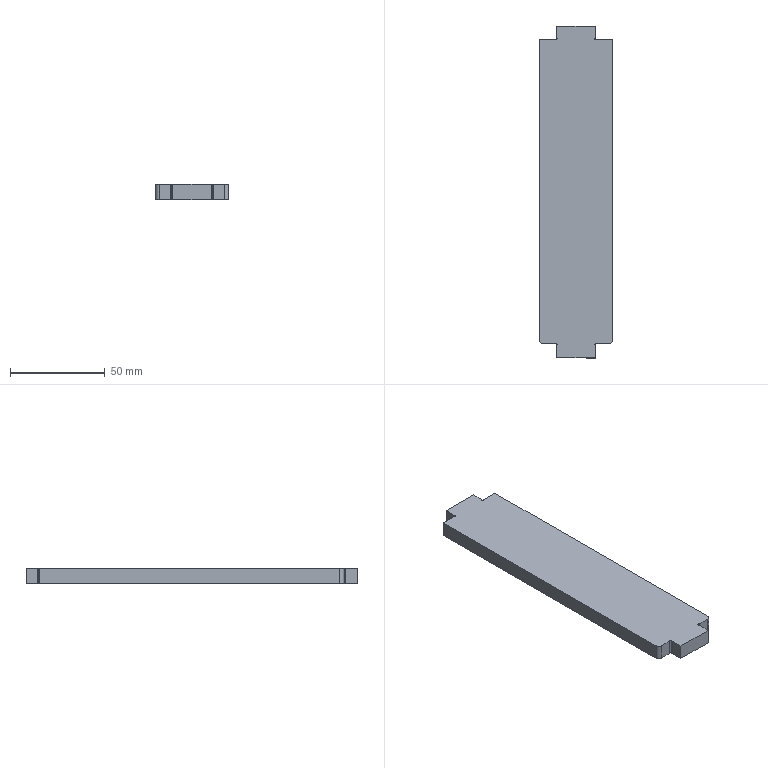Part | SolidWorks | features Fillet 2, FlatPattern 1, ICE 1, SMBaseFlange 1, SheetMetal 1 | 1 solid | 30 faces | box 38.5 x 175.3 x 8 mm | volume 51881 mm3 | cylinder 16 | plane 14 | commonest cylinder face diameters 2 x8 1 x6 4 x2
STEP:
#1=CARTESIAN_POINT('',(110.607,-414.685,0.));
#2=VERTEX_POINT('',#1);
#3=CARTESIAN_POINT('',(109.831,-415.102,0.));
#4=VERTEX_POINT('',#3);
#5=CARTESIAN_POINT('',(110.331,-415.102,0.));
#6=DIRECTION('',(0.,0.,1.));
#7=DIRECTION('',(1.,0.,0.));
#8=AXIS2_PLACEMENT_3D('',#5,#6,#7);
#9=CIRCLE('',#8,0.5);
#10=EDGE_CURVE('',#2,#4,#9,.T.);
#11=ORIENTED_EDGE('',*,*,#10,.T.);
#12=CARTESIAN_POINT('',(109.831,-415.102,-8.));
#13=VERTEX_POINT('',#12);
#14=CARTESIAN_POINT('',(109.831,-415.102,-8.));
#15=DIRECTION('',(0.,0.,-1.));
#16=VECTOR('',#15,1000.);
#17=LINE('',#14,#16);
#18=EDGE_CURVE('',#4,#13,#17,.T.);
#19=ORIENTED_EDGE('',*,*,#18,.T.);
#20=CARTESIAN_POINT('',(110.607,-414.685,-8.));
#21=VERTEX_POINT('',#20);
#22=CARTESIAN_POINT('',(110.331,-415.102,-8.));
#23=DIRECTION('',(0.,0.,1.));
#24=DIRECTION('',(1.,0.,0.));
#25=AXIS2_PLACEMENT_3D('',#22,#23,#24);
#26=CIRCLE('',#25,0.5);
#27=EDGE_CURVE('',#21,#13,#26,.T.);
#28=ORIENTED_EDGE('',*,*,#27,.F.);
#29=CARTESIAN_POINT('',(110.607,-414.685,-8.));
#30=DIRECTION('',(0.,0.,1.));
#31=VECTOR('',#30,1000.);
#32=LINE('',#29,#31);
#33=EDGE_CURVE('',#21,#2,#32,.T.);
#34=ORIENTED_EDGE('',*,*,#33,.T.);
#35=EDGE_LOOP('',(#11,#19,#28,#34));
#36=FACE_OUTER_BOUND('',#35,.T.);
#37=CARTESIAN_POINT('',(110.331,-415.102,-8.));
#38=DIRECTION('',(0.,0.,-1.));
#39=DIRECTION('',(-1.,0.,0.));
#40=AXIS2_PLACEMENT_3D('',#37,#38,#39);
#41=CYLINDRICAL_SURFACE('',#40,0.5);
#42=ADVANCED_FACE('',(#36),#41,.F.);
#43=CARTESIAN_POINT('',(109.914,-253.526,0.));
#44=VERTEX_POINT('',#43);
#45=CARTESIAN_POINT('',(109.831,-253.802,0.));
#46=VERTEX_POINT('',#45);
#47=CARTESIAN_POINT('',(110.331,-253.802,0.));
#48=DIRECTION('',(0.,0.,1.));
#49=DIRECTION('',(1.,0.,0.));
#50=AXIS2_PLACEMENT_3D('',#47,#48,#49);
#51=CIRCLE('',#50,0.5);
#52=EDGE_CURVE('',#44,#46,#51,.T.);
#53=ORIENTED_EDGE('',*,*,#52,.T.);
#54=CARTESIAN_POINT('',(109.831,-253.802,-8.));
#55=VERTEX_POINT('',#54);
#56=CARTESIAN_POINT('',(109.831,-253.802,-8.));
#57=DIRECTION('',(0.,0.,-1.));
#58=VECTOR('',#57,1000.);
#59=LINE('',#56,#58);
#60=EDGE_CURVE('',#46,#55,#59,.T.);
#61=ORIENTED_EDGE('',*,*,#60,.T.);
#62=CARTESIAN_POINT('',(109.914,-253.526,-8.));
#63=VERTEX_POINT('',#62);
#64=CARTESIAN_POINT('',(110.331,-253.802,-8.));
#65=DIRECTION('',(0.,0.,1.));
#66=DIRECTION('',(1.,0.,0.));
#67=AXIS2_PLACEMENT_3D('',#64,#65,#66);
#68=CIRCLE('',#67,0.5);
#69=EDGE_CURVE('',#63,#55,#68,.T.);
#70=ORIENTED_EDGE('',*,*,#69,.F.);
#71=CARTESIAN_POINT('',(109.914,-253.526,-8.));
#72=DIRECTION('',(0.,0.,1.));
#73=VECTOR('',#72,1000.);
#74=LINE('',#71,#73);
#75=EDGE_CURVE('',#63,#44,#74,.T.);
#76=ORIENTED_EDGE('',*,*,#75,.T.);
#77=EDGE_LOOP('',(#53,#61,#70,#76));
#78=FACE_OUTER_BOUND('',#77,.T.);
#79=CARTESIAN_POINT('',(110.331,-253.802,-8.));
#80=DIRECTION('',(0.,0.,-1.));
#81=DIRECTION('',(-1.,0.,0.));
#82=AXIS2_PLACEMENT_3D('',#79,#80,#81);
#83=CYLINDRICAL_SURFACE('',#82,0.5);
#84=ADVANCED_FACE('',(#78),#83,.F.);
#85=CARTESIAN_POINT('',(82.581,-414.852,0.));
#86=VERTEX_POINT('',#85);
#87=CARTESIAN_POINT('',(88.502,-414.852,0.));
#88=VERTEX_POINT('',#87);
#89=CARTESIAN_POINT('',(80.581,-414.852,0.));
#90=DIRECTION('',(1.,0.,0.));
#91=VECTOR('',#90,1000.);
#92=LINE('',#89,#91);
#93=EDGE_CURVE('',#86,#88,#92,.T.);
#94=ORIENTED_EDGE('',*,*,#93,.F.);
#95=CARTESIAN_POINT('',(82.581,-414.852,-8.));
#96=VERTEX_POINT('',#95);
#97=CARTESIAN_POINT('',(82.581,-414.852,-8.));
#98=DIRECTION('',(0.,0.,-1.));
#99=VECTOR('',#98,1000.);
#100=LINE('',#97,#99);
#101=EDGE_CURVE('',#86,#96,#100,.T.);
#102=ORIENTED_EDGE('',*,*,#101,.T.);
#103=CARTESIAN_POINT('',(88.502,-414.852,-8.));
#104=VERTEX_POINT('',#103);
#105=CARTESIAN_POINT('',(80.581,-414.852,-8.));
#106=DIRECTION('',(1.,0.,0.));
#107=VECTOR('',#106,1000.);
#108=LINE('',#105,#107);
#109=EDGE_CURVE('',#96,#104,#108,.T.);
#110=ORIENTED_EDGE('',*,*,#109,.T.);
#111=CARTESIAN_POINT('',(88.502,-414.852,-8.));
#112=DIRECTION('',(0.,0.,1.));
#113=VECTOR('',#112,1000.);
#114=LINE('',#111,#113);
#115=EDGE_CURVE('',#104,#88,#114,.T.);
#116=ORIENTED_EDGE('',*,*,#115,.T.);
#117=EDGE_LOOP('',(#94,#102,#110,#116));
#118=FACE_OUTER_BOUND('',#117,.T.);
#119=CARTESIAN_POINT('',(80.581,-414.852,-8.));
#120=DIRECTION('',(0.,-1.,0.));
#121=DIRECTION('',(1.,0.,0.));
#122=AXIS2_PLACEMENT_3D('',#119,#120,#121);
#123=PLANE('',#122);
#124=ADVANCED_FACE('',(#118),#123,.T.);
#125=CARTESIAN_POINT('',(88.502,-254.052,0.));
#126=VERTEX_POINT('',#125);
#127=CARTESIAN_POINT('',(80.581,-254.052,0.));
#128=VERTEX_POINT('',#127);
#129=CARTESIAN_POINT('',(80.581,-254.052,0.));
#130=DIRECTION('',(-1.,0.,0.));
#131=VECTOR('',#130,1000.);
#132=LINE('',#129,#131);
#133=EDGE_CURVE('',#126,#128,#132,.T.);
#134=ORIENTED_EDGE('',*,*,#133,.F.);
#135=CARTESIAN_POINT('',(88.502,-254.052,-8.));
#136=VERTEX_POINT('',#135);
#137=CARTESIAN_POINT('',(88.502,-254.052,-8.));
#138=DIRECTION('',(0.,0.,-1.));
#139=VECTOR('',#138,1000.);
#140=LINE('',#137,#139);
#141=EDGE_CURVE('',#126,#136,#140,.T.);
#142=ORIENTED_EDGE('',*,*,#141,.T.);
#143=CARTESIAN_POINT('',(80.581,-254.052,-8.));
#144=VERTEX_POINT('',#143);
#145=CARTESIAN_POINT('',(80.581,-254.052,-8.));
#146=DIRECTION('',(-1.,0.,0.));
#147=VECTOR('',#146,1000.);
#148=LINE('',#145,#147);
#149=EDGE_CURVE('',#136,#144,#148,.T.);
#150=ORIENTED_EDGE('',*,*,#149,.T.);
#151=CARTESIAN_POINT('',(80.581,-254.052,-8.));
#152=DIRECTION('',(0.,0.,1.));
#153=VECTOR('',#152,1000.);
#154=LINE('',#151,#153);
#155=EDGE_CURVE('',#144,#128,#154,.T.);
#156=ORIENTED_EDGE('',*,*,#155,.T.);
#157=EDGE_LOOP('',(#134,#142,#150,#156));
#158=FACE_OUTER_BOUND('',#157,.T.);
#159=CARTESIAN_POINT('',(80.581,-254.052,-8.));
#160=DIRECTION('',(0.,1.,0.));
#161=DIRECTION('',(0.,0.,1.));
#162=AXIS2_PLACEMENT_3D('',#159,#160,#161);
#163=PLANE('',#162);
#164=ADVANCED_FACE('',(#158),#163,.T.);
#165=CARTESIAN_POINT('',(89.581,-247.052,-8.));
#166=VERTEX_POINT('',#165);
#167=CARTESIAN_POINT('',(89.581,-252.973,-8.));
#168=VERTEX_POINT('',#167);
#169=CARTESIAN_POINT('',(89.581,-254.052,-8.));
#170=DIRECTION('',(0.,-1.,0.));
#171=VECTOR('',#170,1000.);
#172=LINE('',#169,#171);
#173=EDGE_CURVE('',#166,#168,#172,.T.);
#174=ORIENTED_EDGE('',*,*,#173,.T.);
#175=CARTESIAN_POINT('',(89.581,-252.973,0.));
#176=VERTEX_POINT('',#175);
#177=CARTESIAN_POINT('',(89.581,-252.973,-8.));
#178=DIRECTION('',(0.,0.,1.));
#179=VECTOR('',#178,1000.);
#180=LINE('',#177,#179);
#181=EDGE_CURVE('',#168,#176,#180,.T.);
#182=ORIENTED_EDGE('',*,*,#181,.T.);
#183=CARTESIAN_POINT('',(89.581,-247.052,0.));
#184=VERTEX_POINT('',#183);
#185=CARTESIAN_POINT('',(89.581,-254.052,0.));
#186=DIRECTION('',(0.,-1.,0.));
#187=VECTOR('',#186,1000.);
#188=LINE('',#185,#187);
#189=EDGE_CURVE('',#184,#176,#188,.T.);
#190=ORIENTED_EDGE('',*,*,#189,.F.);
#191=CARTESIAN_POINT('',(89.581,-247.052,-8.));
#192=DIRECTION('',(0.,0.,1.));
#193=VECTOR('',#192,1000.);
#194=LINE('',#191,#193);
#195=EDGE_CURVE('',#166,#184,#194,.T.);
#196=ORIENTED_EDGE('',*,*,#195,.F.);
#197=EDGE_LOOP('',(#174,#182,#190,#196));
#198=FACE_OUTER_BOUND('',#197,.T.);
#199=CARTESIAN_POINT('',(89.581,-254.052,-8.));
#200=DIRECTION('',(-1.,0.,0.));
#201=DIRECTION('',(0.,0.,1.));
#202=AXIS2_PLACEMENT_3D('',#199,#200,#201);
#203=PLANE('',#202);
#204=ADVANCED_FACE('',(#198),#203,.T.);
#205=CARTESIAN_POINT('',(110.081,-252.973,0.));
#206=VERTEX_POINT('',#205);
#207=CARTESIAN_POINT('',(110.081,-247.052,0.));
#208=VERTEX_POINT('',#207);
#209=CARTESIAN_POINT('',(110.081,-247.052,0.));
#210=DIRECTION('',(0.,1.,0.));
#211=VECTOR('',#210,1000.);
#212=LINE('',#209,#211);
#213=EDGE_CURVE('',#206,#208,#212,.T.);
#214=ORIENTED_EDGE('',*,*,#213,.F.);
#215=CARTESIAN_POINT('',(110.081,-252.973,-8.));
#216=VERTEX_POINT('',#215);
#217=CARTESIAN_POINT('',(110.081,-252.973,-8.));
#218=DIRECTION('',(0.,0.,-1.));
#219=VECTOR('',#218,1000.);
#220=LINE('',#217,#219);
#221=EDGE_CURVE('',#206,#216,#220,.T.);
#222=ORIENTED_EDGE('',*,*,#221,.T.);
#223=CARTESIAN_POINT('',(110.081,-247.052,-8.));
#224=VERTEX_POINT('',#223);
#225=CARTESIAN_POINT('',(110.081,-247.052,-8.));
#226=DIRECTION('',(0.,1.,0.));
#227=VECTOR('',#226,1000.);
#228=LINE('',#225,#227);
#229=EDGE_CURVE('',#216,#224,#228,.T.);
#230=ORIENTED_EDGE('',*,*,#229,.T.);
#231=CARTESIAN_POINT('',(110.081,-247.052,-8.));
#232=DIRECTION('',(0.,0.,1.));
#233=VECTOR('',#232,1000.);
#234=LINE('',#231,#233);
#235=EDGE_CURVE('',#224,#208,#234,.T.);
#236=ORIENTED_EDGE('',*,*,#235,.T.);
#237=EDGE_LOOP('',(#214,#222,#230,#236));
#238=FACE_OUTER_BOUND('',#237,.T.);
#239=CARTESIAN_POINT('',(110.081,-247.052,-8.));
#240=DIRECTION('',(1.,0.,0.));
#241=DIRECTION('',(0.,0.,-1.));
#242=AXIS2_PLACEMENT_3D('',#239,#240,#241);
#243=PLANE('',#242);
#244=ADVANCED_FACE('',(#238),#243,.T.);
#245=CARTESIAN_POINT('',(119.081,-254.052,-8.));
#246=VERTEX_POINT('',#245);
#247=CARTESIAN_POINT('',(111.16,-254.052,-8.));
#248=VERTEX_POINT('',#247);
#249=CARTESIAN_POINT('',(110.081,-254.052,-8.));
#250=DIRECTION('',(-1.,0.,0.));
#251=VECTOR('',#250,1000.);
#252=LINE('',#249,#251);
#253=EDGE_CURVE('',#246,#248,#252,.T.);
#254=ORIENTED_EDGE('',*,*,#253,.T.);
#255=CARTESIAN_POINT('',(111.16,-254.052,0.));
#256=VERTEX_POINT('',#255);
#257=CARTESIAN_POINT('',(111.16,-254.052,-8.));
#258=DIRECTION('',(0.,0.,1.));
#259=VECTOR('',#258,1000.);
#260=LINE('',#257,#259);
#261=EDGE_CURVE('',#248,#256,#260,.T.);
#262=ORIENTED_EDGE('',*,*,#261,.T.);
#263=CARTESIAN_POINT('',(119.081,-254.052,0.));
#264=VERTEX_POINT('',#263);
#265=CARTESIAN_POINT('',(110.081,-254.052,0.));
#266=DIRECTION('',(-1.,0.,0.));
#267=VECTOR('',#266,1000.);
#268=LINE('',#265,#267);
#269=EDGE_CURVE('',#264,#256,#268,.T.);
#270=ORIENTED_EDGE('',*,*,#269,.F.);
#271=CARTESIAN_POINT('',(119.081,-254.052,-8.));
#272=DIRECTION('',(0.,0.,1.));
#273=VECTOR('',#272,1000.);
#274=LINE('',#271,#273);
#275=EDGE_CURVE('',#246,#264,#274,.T.);
#276=ORIENTED_EDGE('',*,*,#275,.F.);
#277=EDGE_LOOP('',(#254,#262,#270,#276));
#278=FACE_OUTER_BOUND('',#277,.T.);
#279=CARTESIAN_POINT('',(110.081,-254.052,-8.));
#280=DIRECTION('',(0.,1.,0.));
#281=DIRECTION('',(0.,0.,1.));
#282=AXIS2_PLACEMENT_3D('',#279,#280,#281);
#283=PLANE('',#282);
#284=ADVANCED_FACE('',(#278),#283,.T.);
#285=CARTESIAN_POINT('',(111.16,-414.852,-8.));
#286=VERTEX_POINT('',#285);
#287=CARTESIAN_POINT('',(117.081,-414.852,-8.));
#288=VERTEX_POINT('',#287);
#289=CARTESIAN_POINT('',(110.081,-414.852,-8.));
#290=DIRECTION('',(1.,0.,0.));
#291=VECTOR('',#290,1000.);
#292=LINE('',#289,#291);
#293=EDGE_CURVE('',#286,#288,#292,.T.);
#294=ORIENTED_EDGE('',*,*,#293,.T.);
#295=CARTESIAN_POINT('',(117.081,-414.852,0.));
#296=VERTEX_POINT('',#295);
#297=CARTESIAN_POINT('',(117.081,-414.852,-8.));
#298=DIRECTION('',(0.,0.,1.));
#299=VECTOR('',#298,1000.);
#300=LINE('',#297,#299);
#301=EDGE_CURVE('',#288,#296,#300,.T.);
#302=ORIENTED_EDGE('',*,*,#301,.T.);
#303=CARTESIAN_POINT('',(111.16,-414.852,0.));
#304=VERTEX_POINT('',#303);
#305=CARTESIAN_POINT('',(110.081,-414.852,0.));
#306=DIRECTION('',(1.,0.,0.));
#307=VECTOR('',#306,1000.);
#308=LINE('',#305,#307);
#309=EDGE_CURVE('',#304,#296,#308,.T.);
#310=ORIENTED_EDGE('',*,*,#309,.F.);
#311=CARTESIAN_POINT('',(111.16,-414.852,-8.));
#312=DIRECTION('',(0.,0.,-1.));
#313=VECTOR('',#312,1000.);
#314=LINE('',#311,#313);
#315=EDGE_CURVE('',#304,#286,#314,.T.);
#316=ORIENTED_EDGE('',*,*,#315,.T.);
#317=EDGE_LOOP('',(#294,#302,#310,#316));
#318=FACE_OUTER_BOUND('',#317,.T.);
#319=CARTESIAN_POINT('',(110.081,-414.852,-8.));
#320=DIRECTION('',(0.,-1.,0.));
#321=DIRECTION('',(1.,0.,0.));
#322=AXIS2_PLACEMENT_3D('',#319,#320,#321);
#323=PLANE('',#322);
#324=ADVANCED_FACE('',(#318),#323,.T.);
#325=CARTESIAN_POINT('',(110.081,-422.352,-8.));
#326=VERTEX_POINT('',#325);
#327=CARTESIAN_POINT('',(110.081,-415.931,-8.));
#328=VERTEX_POINT('',#327);
#329=CARTESIAN_POINT('',(110.081,-422.352,-8.));
#330=DIRECTION('',(0.,1.,0.));
#331=VECTOR('',#330,1000.);
#332=LINE('',#329,#331);
#333=EDGE_CURVE('',#326,#328,#332,.T.);
#334=ORIENTED_EDGE('',*,*,#333,.T.);
#335=CARTESIAN_POINT('',(110.081,-415.931,0.));
#336=VERTEX_POINT('',#335);
#337=CARTESIAN_POINT('',(110.081,-415.931,-8.));
#338=DIRECTION('',(0.,0.,1.));
#339=VECTOR('',#338,1000.);
#340=LINE('',#337,#339);
#341=EDGE_CURVE('',#328,#336,#340,.T.);
#342=ORIENTED_EDGE('',*,*,#341,.T.);
#343=CARTESIAN_POINT('',(110.081,-422.352,0.));
#344=VERTEX_POINT('',#343);
#345=CARTESIAN_POINT('',(110.081,-422.352,0.));
#346=DIRECTION('',(0.,1.,0.));
#347=VECTOR('',#346,1000.);
#348=LINE('',#345,#347);
#349=EDGE_CURVE('',#344,#336,#348,.T.);
#350=ORIENTED_EDGE('',*,*,#349,.F.);
#351=CARTESIAN_POINT('',(110.081,-422.352,-8.));
#352=DIRECTION('',(0.,0.,1.));
#353=VECTOR('',#352,1000.);
#354=LINE('',#351,#353);
#355=EDGE_CURVE('',#326,#344,#354,.T.);
#356=ORIENTED_EDGE('',*,*,#355,.F.);
#357=EDGE_LOOP('',(#334,#342,#350,#356));
#358=FACE_OUTER_BOUND('',#357,.T.);
#359=CARTESIAN_POINT('',(110.081,-422.352,-8.));
#360=DIRECTION('',(1.,0.,0.));
#361=DIRECTION('',(0.,0.,-1.));
#362=AXIS2_PLACEMENT_3D('',#359,#360,#361);
#363=PLANE('',#362);
#364=ADVANCED_FACE('',(#358),#363,.T.);
#365=CARTESIAN_POINT('',(89.581,-415.931,0.));
#366=VERTEX_POINT('',#365);
#367=CARTESIAN_POINT('',(89.581,-422.352,0.));
#368=VERTEX_POINT('',#367);
#369=CARTESIAN_POINT('',(89.581,-414.852,0.));
#370=DIRECTION('',(0.,-1.,0.));
#371=VECTOR('',#370,1000.);
#372=LINE('',#369,#371);
#373=EDGE_CURVE('',#366,#368,#372,.T.);
#374=ORIENTED_EDGE('',*,*,#373,.F.);
#375=CARTESIAN_POINT('',(89.581,-415.931,-8.));
#376=VERTEX_POINT('',#375);
#377=CARTESIAN_POINT('',(89.581,-415.931,-8.));
#378=DIRECTION('',(0.,0.,-1.));
#379=VECTOR('',#378,1000.);
#380=LINE('',#377,#379);
#381=EDGE_CURVE('',#366,#376,#380,.T.);
#382=ORIENTED_EDGE('',*,*,#381,.T.);
#383=CARTESIAN_POINT('',(89.581,-422.352,-8.));
#384=VERTEX_POINT('',#383);
#385=CARTESIAN_POINT('',(89.581,-414.852,-8.));
#386=DIRECTION('',(0.,-1.,0.));
#387=VECTOR('',#386,1000.);
#388=LINE('',#385,#387);
#389=EDGE_CURVE('',#376,#384,#388,.T.);
#390=ORIENTED_EDGE('',*,*,#389,.T.);
#391=CARTESIAN_POINT('',(89.581,-422.352,-8.));
#392=DIRECTION('',(0.,0.,1.));
#393=VECTOR('',#392,1000.);
#394=LINE('',#391,#393);
#395=EDGE_CURVE('',#384,#368,#394,.T.);
#396=ORIENTED_EDGE('',*,*,#395,.T.);
#397=EDGE_LOOP('',(#374,#382,#390,#396));
#398=FACE_OUTER_BOUND('',#397,.T.);
#399=CARTESIAN_POINT('',(89.581,-414.852,-8.));
#400=DIRECTION('',(-1.,0.,0.));
#401=DIRECTION('',(0.,-1.,0.));
#402=AXIS2_PLACEMENT_3D('',#399,#400,#401);
#403=PLANE('',#402);
#404=ADVANCED_FACE('',(#398),#403,.T.);
#405=CARTESIAN_POINT('',(119.081,-412.852,-8.));
#406=VERTEX_POINT('',#405);
#407=CARTESIAN_POINT('',(119.081,-254.052,-8.));
#408=DIRECTION('',(0.,1.,0.));
#409=VECTOR('',#408,1000.);
#410=LINE('',#407,#409);
#411=EDGE_CURVE('',#406,#246,#410,.T.);
#412=ORIENTED_EDGE('',*,*,#411,.F.);
#413=CARTESIAN_POINT('',(117.081,-412.852,-8.));
#414=DIRECTION('',(0.,0.,-1.));
#415=DIRECTION('',(-1.,0.,0.));
#416=AXIS2_PLACEMENT_3D('',#413,#414,#415);
#417=CIRCLE('',#416,2.);
#418=EDGE_CURVE('',#406,#288,#417,.T.);
#419=ORIENTED_EDGE('',*,*,#418,.T.);
#420=ORIENTED_EDGE('',*,*,#293,.F.);
#421=CARTESIAN_POINT('',(111.16,-413.852,-8.));
#422=DIRECTION('',(0.,0.,-1.));
#423=DIRECTION('',(-1.,0.,0.));
#424=AXIS2_PLACEMENT_3D('',#421,#422,#423);
#425=CIRCLE('',#424,1.);
#426=EDGE_CURVE('',#286,#21,#425,.T.);
#427=ORIENTED_EDGE('',*,*,#426,.T.);
#428=ORIENTED_EDGE('',*,*,#27,.T.);
#429=CARTESIAN_POINT('',(109.914,-415.378,-8.));
#430=VERTEX_POINT('',#429);
#431=CARTESIAN_POINT('',(110.331,-415.102,-8.));
#432=DIRECTION('',(0.,0.,1.));
#433=DIRECTION('',(1.,0.,0.));
#434=AXIS2_PLACEMENT_3D('',#431,#432,#433);
#435=CIRCLE('',#434,0.5);
#436=EDGE_CURVE('',#13,#430,#435,.T.);
#437=ORIENTED_EDGE('',*,*,#436,.T.);
#438=CARTESIAN_POINT('',(109.081,-415.931,-8.));
#439=DIRECTION('',(0.,0.,-1.));
#440=DIRECTION('',(-1.,0.,0.));
#441=AXIS2_PLACEMENT_3D('',#438,#439,#440);
#442=CIRCLE('',#441,1.);
#443=EDGE_CURVE('',#430,#328,#442,.T.);
#444=ORIENTED_EDGE('',*,*,#443,.T.);
#445=ORIENTED_EDGE('',*,*,#333,.F.);
#446=CARTESIAN_POINT('',(89.581,-422.352,-8.));
#447=DIRECTION('',(1.,0.,0.));
#448=VECTOR('',#447,1000.);
#449=LINE('',#446,#448);
#450=EDGE_CURVE('',#384,#326,#449,.T.);
#451=ORIENTED_EDGE('',*,*,#450,.F.);
#452=ORIENTED_EDGE('',*,*,#389,.F.);
#453=CARTESIAN_POINT('',(89.747,-415.378,-8.));
#454=VERTEX_POINT('',#453);
#455=CARTESIAN_POINT('',(90.581,-415.931,-8.));
#456=DIRECTION('',(0.,0.,-1.));
#457=DIRECTION('',(-1.,0.,0.));
#458=AXIS2_PLACEMENT_3D('',#455,#456,#457);
#459=CIRCLE('',#458,1.);
#460=EDGE_CURVE('',#376,#454,#459,.T.);
#461=ORIENTED_EDGE('',*,*,#460,.T.);
#462=CARTESIAN_POINT('',(89.054,-414.685,-8.));
#463=VERTEX_POINT('',#462);
#464=CARTESIAN_POINT('',(89.331,-415.102,-8.));
#465=DIRECTION('',(0.,0.,-1.));
#466=DIRECTION('',(-1.,0.,0.));
#467=AXIS2_PLACEMENT_3D('',#464,#465,#466);
#468=CIRCLE('',#467,0.5);
#469=EDGE_CURVE('',#463,#454,#468,.T.);
#470=ORIENTED_EDGE('',*,*,#469,.F.);
#471=CARTESIAN_POINT('',(88.502,-413.852,-8.));
#472=DIRECTION('',(0.,0.,-1.));
#473=DIRECTION('',(-1.,0.,0.));
#474=AXIS2_PLACEMENT_3D('',#471,#472,#473);
#475=CIRCLE('',#474,1.);
#476=EDGE_CURVE('',#463,#104,#475,.T.);
#477=ORIENTED_EDGE('',*,*,#476,.T.);
#478=ORIENTED_EDGE('',*,*,#109,.F.);
#479=CARTESIAN_POINT('',(80.581,-412.852,-8.));
#480=VERTEX_POINT('',#479);
#481=CARTESIAN_POINT('',(82.581,-412.852,-8.));
#482=DIRECTION('',(0.,0.,-1.));
#483=DIRECTION('',(-1.,0.,0.));
#484=AXIS2_PLACEMENT_3D('',#481,#482,#483);
#485=CIRCLE('',#484,2.);
#486=EDGE_CURVE('',#96,#480,#485,.T.);
#487=ORIENTED_EDGE('',*,*,#486,.T.);
#488=CARTESIAN_POINT('',(80.581,-414.852,-8.));
#489=DIRECTION('',(0.,-1.,0.));
#490=VECTOR('',#489,1000.);
#491=LINE('',#488,#490);
#492=EDGE_CURVE('',#144,#480,#491,.T.);
#493=ORIENTED_EDGE('',*,*,#492,.F.);
#494=ORIENTED_EDGE('',*,*,#149,.F.);
#495=CARTESIAN_POINT('',(89.054,-254.219,-8.));
#496=VERTEX_POINT('',#495);
#497=CARTESIAN_POINT('',(88.502,-255.052,-8.));
#498=DIRECTION('',(0.,0.,-1.));
#499=DIRECTION('',(-1.,0.,0.));
#500=AXIS2_PLACEMENT_3D('',#497,#498,#499);
#501=CIRCLE('',#500,1.);
#502=EDGE_CURVE('',#136,#496,#501,.T.);
#503=ORIENTED_EDGE('',*,*,#502,.T.);
#504=CARTESIAN_POINT('',(89.747,-253.526,-8.));
#505=VERTEX_POINT('',#504);
#506=CARTESIAN_POINT('',(89.331,-253.802,-8.));
#507=DIRECTION('',(0.,0.,1.));
#508=DIRECTION('',(1.,0.,0.));
#509=AXIS2_PLACEMENT_3D('',#506,#507,#508);
#510=CIRCLE('',#509,0.5);
#511=EDGE_CURVE('',#496,#505,#510,.T.);
#512=ORIENTED_EDGE('',*,*,#511,.T.);
#513=CARTESIAN_POINT('',(90.581,-252.973,-8.));
#514=DIRECTION('',(0.,0.,-1.));
#515=DIRECTION('',(-1.,0.,0.));
#516=AXIS2_PLACEMENT_3D('',#513,#514,#515);
#517=CIRCLE('',#516,1.);
#518=EDGE_CURVE('',#505,#168,#517,.T.);
#519=ORIENTED_EDGE('',*,*,#518,.T.);
#520=ORIENTED_EDGE('',*,*,#173,.F.);
#521=CARTESIAN_POINT('',(89.581,-247.052,-8.));
#522=DIRECTION('',(-1.,0.,0.));
#523=VECTOR('',#522,1000.);
#524=LINE('',#521,#523);
#525=EDGE_CURVE('',#224,#166,#524,.T.);
#526=ORIENTED_EDGE('',*,*,#525,.F.);
#527=ORIENTED_EDGE('',*,*,#229,.F.);
#528=CARTESIAN_POINT('',(109.081,-252.973,-8.));
#529=DIRECTION('',(0.,0.,-1.));
#530=DIRECTION('',(-1.,0.,0.));
#531=AXIS2_PLACEMENT_3D('',#528,#529,#530);
#532=CIRCLE('',#531,1.);
#533=EDGE_CURVE('',#216,#63,#532,.T.);
#534=ORIENTED_EDGE('',*,*,#533,.T.);
#535=ORIENTED_EDGE('',*,*,#69,.T.);
#536=CARTESIAN_POINT('',(110.607,-254.219,-8.));
#537=VERTEX_POINT('',#536);
#538=CARTESIAN_POINT('',(110.331,-253.802,-8.));
#539=DIRECTION('',(0.,0.,1.));
#540=DIRECTION('',(1.,0.,0.));
#541=AXIS2_PLACEMENT_3D('',#538,#539,#540);
#542=CIRCLE('',#541,0.5);
#543=EDGE_CURVE('',#55,#537,#542,.T.);
#544=ORIENTED_EDGE('',*,*,#543,.T.);
#545=CARTESIAN_POINT('',(111.16,-255.052,-8.));
#546=DIRECTION('',(0.,0.,-1.));
#547=DIRECTION('',(-1.,0.,0.));
#548=AXIS2_PLACEMENT_3D('',#545,#546,#547);
#549=CIRCLE('',#548,1.);
#550=EDGE_CURVE('',#537,#248,#549,.T.);
#551=ORIENTED_EDGE('',*,*,#550,.T.);
#552=ORIENTED_EDGE('',*,*,#253,.F.);
#553=EDGE_LOOP('',(#412,#419,#420,#427,#428,#437,#444,#445,#451,#452,#461,#470,#477,#478,#487,#493,#494,#503,#512,#519,#520,#526,#527,#534,#535,#544,#551,#552));
#554=FACE_OUTER_BOUND('',#553,.T.);
#555=CARTESIAN_POINT('',(0.,0.,-8.));
#556=DIRECTION('',(0.,0.,-1.));
#557=DIRECTION('',(-1.,0.,0.));
#558=AXIS2_PLACEMENT_3D('',#555,#556,#557);
#559=PLANE('',#558);
#560=ADVANCED_FACE('',(#554),#559,.T.);
#561=ORIENTED_EDGE('',*,*,#309,.T.);
#562=CARTESIAN_POINT('',(119.081,-412.852,0.));
#563=VERTEX_POINT('',#562);
#564=CARTESIAN_POINT('',(117.081,-412.852,0.));
#565=DIRECTION('',(0.,0.,1.));
#566=DIRECTION('',(-1.,0.,0.));
#567=AXIS2_PLACEMENT_3D('',#564,#565,#566);
#568=CIRCLE('',#567,2.);
#569=EDGE_CURVE('',#296,#563,#568,.T.);
#570=ORIENTED_EDGE('',*,*,#569,.T.);
#571=CARTESIAN_POINT('',(119.081,-254.052,0.));
#572=DIRECTION('',(0.,1.,0.));
#573=VECTOR('',#572,1000.);
#574=LINE('',#571,#573);
#575=EDGE_CURVE('',#563,#264,#574,.T.);
#576=ORIENTED_EDGE('',*,*,#575,.T.);
#577=ORIENTED_EDGE('',*,*,#269,.T.);
#578=CARTESIAN_POINT('',(110.607,-254.219,0.));
#579=VERTEX_POINT('',#578);
#580=CARTESIAN_POINT('',(111.16,-255.052,0.));
#581=DIRECTION('',(0.,0.,1.));
#582=DIRECTION('',(-1.,0.,0.));
#583=AXIS2_PLACEMENT_3D('',#580,#581,#582);
#584=CIRCLE('',#583,1.);
#585=EDGE_CURVE('',#256,#579,#584,.T.);
#586=ORIENTED_EDGE('',*,*,#585,.T.);
#587=CARTESIAN_POINT('',(110.331,-253.802,0.));
#588=DIRECTION('',(0.,0.,1.));
#589=DIRECTION('',(1.,0.,0.));
#590=AXIS2_PLACEMENT_3D('',#587,#588,#589);
#591=CIRCLE('',#590,0.5);
#592=EDGE_CURVE('',#46,#579,#591,.T.);
#593=ORIENTED_EDGE('',*,*,#592,.F.);
#594=ORIENTED_EDGE('',*,*,#52,.F.);
#595=CARTESIAN_POINT('',(109.081,-252.973,0.));
#596=DIRECTION('',(0.,0.,1.));
#597=DIRECTION('',(-1.,0.,0.));
#598=AXIS2_PLACEMENT_3D('',#595,#596,#597);
#599=CIRCLE('',#598,1.);
#600=EDGE_CURVE('',#44,#206,#599,.T.);
#601=ORIENTED_EDGE('',*,*,#600,.T.);
#602=ORIENTED_EDGE('',*,*,#213,.T.);
#603=CARTESIAN_POINT('',(89.581,-247.052,0.));
#604=DIRECTION('',(-1.,0.,0.));
#605=VECTOR('',#604,1000.);
#606=LINE('',#603,#605);
#607=EDGE_CURVE('',#208,#184,#606,.T.);
#608=ORIENTED_EDGE('',*,*,#607,.T.);
#609=ORIENTED_EDGE('',*,*,#189,.T.);
#610=CARTESIAN_POINT('',(89.747,-253.526,0.));
#611=VERTEX_POINT('',#610);
#612=CARTESIAN_POINT('',(90.581,-252.973,0.));
#613=DIRECTION('',(0.,0.,1.));
#614=DIRECTION('',(-1.,0.,0.));
#615=AXIS2_PLACEMENT_3D('',#612,#613,#614);
#616=CIRCLE('',#615,1.);
#617=EDGE_CURVE('',#176,#611,#616,.T.);
#618=ORIENTED_EDGE('',*,*,#617,.T.);
#619=CARTESIAN_POINT('',(89.054,-254.219,0.));
#620=VERTEX_POINT('',#619);
#621=CARTESIAN_POINT('',(89.331,-253.802,0.));
#622=DIRECTION('',(0.,0.,1.));
#623=DIRECTION('',(1.,0.,0.));
#624=AXIS2_PLACEMENT_3D('',#621,#622,#623);
#625=CIRCLE('',#624,0.5);
#626=EDGE_CURVE('',#620,#611,#625,.T.);
#627=ORIENTED_EDGE('',*,*,#626,.F.);
#628=CARTESIAN_POINT('',(88.502,-255.052,0.));
#629=DIRECTION('',(0.,0.,1.));
#630=DIRECTION('',(-1.,0.,0.));
#631=AXIS2_PLACEMENT_3D('',#628,#629,#630);
#632=CIRCLE('',#631,1.);
#633=EDGE_CURVE('',#620,#126,#632,.T.);
#634=ORIENTED_EDGE('',*,*,#633,.T.);
#635=ORIENTED_EDGE('',*,*,#133,.T.);
#636=CARTESIAN_POINT('',(80.581,-412.852,0.));
#637=VERTEX_POINT('',#636);
#638=CARTESIAN_POINT('',(80.581,-414.852,0.));
#639=DIRECTION('',(0.,-1.,0.));
#640=VECTOR('',#639,1000.);
#641=LINE('',#638,#640);
#642=EDGE_CURVE('',#128,#637,#641,.T.);
#643=ORIENTED_EDGE('',*,*,#642,.T.);
#644=CARTESIAN_POINT('',(82.581,-412.852,0.));
#645=DIRECTION('',(0.,0.,1.));
#646=DIRECTION('',(-1.,0.,0.));
#647=AXIS2_PLACEMENT_3D('',#644,#645,#646);
#648=CIRCLE('',#647,2.);
#649=EDGE_CURVE('',#637,#86,#648,.T.);
#650=ORIENTED_EDGE('',*,*,#649,.T.);
#651=ORIENTED_EDGE('',*,*,#93,.T.);
#652=CARTESIAN_POINT('',(89.054,-414.685,0.));
#653=VERTEX_POINT('',#652);
#654=CARTESIAN_POINT('',(88.502,-413.852,0.));
#655=DIRECTION('',(0.,0.,1.));
#656=DIRECTION('',(-1.,0.,0.));
#657=AXIS2_PLACEMENT_3D('',#654,#655,#656);
#658=CIRCLE('',#657,1.);
#659=EDGE_CURVE('',#88,#653,#658,.T.);
#660=ORIENTED_EDGE('',*,*,#659,.T.);
#661=CARTESIAN_POINT('',(89.747,-415.378,0.));
#662=VERTEX_POINT('',#661);
#663=CARTESIAN_POINT('',(89.331,-415.102,0.));
#664=DIRECTION('',(0.,0.,-1.));
#665=DIRECTION('',(-1.,0.,0.));
#666=AXIS2_PLACEMENT_3D('',#663,#664,#665);
#667=CIRCLE('',#666,0.5);
#668=EDGE_CURVE('',#653,#662,#667,.T.);
#669=ORIENTED_EDGE('',*,*,#668,.T.);
#670=CARTESIAN_POINT('',(90.581,-415.931,0.));
#671=DIRECTION('',(0.,0.,1.));
#672=DIRECTION('',(-1.,0.,0.));
#673=AXIS2_PLACEMENT_3D('',#670,#671,#672);
#674=CIRCLE('',#673,1.);
#675=EDGE_CURVE('',#662,#366,#674,.T.);
#676=ORIENTED_EDGE('',*,*,#675,.T.);
#677=ORIENTED_EDGE('',*,*,#373,.T.);
#678=CARTESIAN_POINT('',(89.581,-422.352,0.));
#679=DIRECTION('',(1.,0.,0.));
#680=VECTOR('',#679,1000.);
#681=LINE('',#678,#680);
#682=EDGE_CURVE('',#368,#344,#681,.T.);
#683=ORIENTED_EDGE('',*,*,#682,.T.);
#684=ORIENTED_EDGE('',*,*,#349,.T.);
#685=CARTESIAN_POINT('',(109.914,-415.378,0.));
#686=VERTEX_POINT('',#685);
#687=CARTESIAN_POINT('',(109.081,-415.931,0.));
#688=DIRECTION('',(0.,0.,1.));
#689=DIRECTION('',(-1.,0.,0.));
#690=AXIS2_PLACEMENT_3D('',#687,#688,#689);
#691=CIRCLE('',#690,1.);
#692=EDGE_CURVE('',#336,#686,#691,.T.);
#693=ORIENTED_EDGE('',*,*,#692,.T.);
#694=CARTESIAN_POINT('',(110.331,-415.102,0.));
#695=DIRECTION('',(0.,0.,1.));
#696=DIRECTION('',(1.,0.,0.));
#697=AXIS2_PLACEMENT_3D('',#694,#695,#696);
#698=CIRCLE('',#697,0.5);
#699=EDGE_CURVE('',#4,#686,#698,.T.);
#700=ORIENTED_EDGE('',*,*,#699,.F.);
#701=ORIENTED_EDGE('',*,*,#10,.F.);
#702=CARTESIAN_POINT('',(111.16,-413.852,0.));
#703=DIRECTION('',(0.,0.,1.));
#704=DIRECTION('',(-1.,0.,0.));
#705=AXIS2_PLACEMENT_3D('',#702,#703,#704);
#706=CIRCLE('',#705,1.);
#707=EDGE_CURVE('',#2,#304,#706,.T.);
#708=ORIENTED_EDGE('',*,*,#707,.T.);
#709=EDGE_LOOP('',(#561,#570,#576,#577,#586,#593,#594,#601,#602,#608,#609,#618,#627,#634,#635,#643,#650,#651,#660,#669,#676,#677,#683,#684,#693,#700,#701,#708));
#710=FACE_OUTER_BOUND('',#709,.T.);
#711=CARTESIAN_POINT('',(0.,0.,0.));
#712=DIRECTION('',(0.,0.,-1.));
#713=DIRECTION('',(-1.,0.,0.));
#714=AXIS2_PLACEMENT_3D('',#711,#712,#713);
#715=PLANE('',#714);
#716=ADVANCED_FACE('',(#710),#715,.F.);
#717=ORIENTED_EDGE('',*,*,#492,.T.);
#718=CARTESIAN_POINT('',(80.581,-412.852,-8.));
#719=DIRECTION('',(0.,0.,1.));
#720=VECTOR('',#719,1000.);
#721=LINE('',#718,#720);
#722=EDGE_CURVE('',#480,#637,#721,.T.);
#723=ORIENTED_EDGE('',*,*,#722,.T.);
#724=ORIENTED_EDGE('',*,*,#642,.F.);
#725=ORIENTED_EDGE('',*,*,#155,.F.);
#726=EDGE_LOOP('',(#717,#723,#724,#725));
#727=FACE_OUTER_BOUND('',#726,.T.);
#728=CARTESIAN_POINT('',(80.581,-414.852,-8.));
#729=DIRECTION('',(-1.,0.,0.));
#730=DIRECTION('',(0.,-1.,0.));
#731=AXIS2_PLACEMENT_3D('',#728,#729,#730);
#732=PLANE('',#731);
#733=ADVANCED_FACE('',(#727),#732,.T.);
#734=ORIENTED_EDGE('',*,*,#607,.F.);
#735=ORIENTED_EDGE('',*,*,#235,.F.);
#736=ORIENTED_EDGE('',*,*,#525,.T.);
#737=ORIENTED_EDGE('',*,*,#195,.T.);
#738=EDGE_LOOP('',(#734,#735,#736,#737));
#739=FACE_OUTER_BOUND('',#738,.T.);
#740=CARTESIAN_POINT('',(89.581,-247.052,-8.));
#741=DIRECTION('',(0.,1.,0.));
#742=DIRECTION('',(0.,0.,1.));
#743=AXIS2_PLACEMENT_3D('',#740,#741,#742);
#744=PLANE('',#743);
#745=ADVANCED_FACE('',(#739),#744,.T.);
#746=ORIENTED_EDGE('',*,*,#575,.F.);
#747=CARTESIAN_POINT('',(119.081,-412.852,-8.));
#748=DIRECTION('',(0.,0.,-1.));
#749=VECTOR('',#748,1000.);
#750=LINE('',#747,#749);
#751=EDGE_CURVE('',#563,#406,#750,.T.);
#752=ORIENTED_EDGE('',*,*,#751,.T.);
#753=ORIENTED_EDGE('',*,*,#411,.T.);
#754=ORIENTED_EDGE('',*,*,#275,.T.);
#755=EDGE_LOOP('',(#746,#752,#753,#754));
#756=FACE_OUTER_BOUND('',#755,.T.);
#757=CARTESIAN_POINT('',(119.081,-254.052,-8.));
#758=DIRECTION('',(1.,0.,0.));
#759=DIRECTION('',(0.,1.,0.));
#760=AXIS2_PLACEMENT_3D('',#757,#758,#759);
#761=PLANE('',#760);
#762=ADVANCED_FACE('',(#756),#761,.T.);
#763=ORIENTED_EDGE('',*,*,#682,.F.);
#764=ORIENTED_EDGE('',*,*,#395,.F.);
#765=ORIENTED_EDGE('',*,*,#450,.T.);
#766=ORIENTED_EDGE('',*,*,#355,.T.);
#767=EDGE_LOOP('',(#763,#764,#765,#766));
#768=FACE_OUTER_BOUND('',#767,.T.);
#769=CARTESIAN_POINT('',(89.581,-422.352,-8.));
#770=DIRECTION('',(0.,-1.,0.));
#771=DIRECTION('',(1.,0.,0.));
#772=AXIS2_PLACEMENT_3D('',#769,#770,#771);
#773=PLANE('',#772);
#774=ADVANCED_FACE('',(#768),#773,.T.);
#775=ORIENTED_EDGE('',*,*,#668,.F.);
#776=CARTESIAN_POINT('',(89.054,-414.685,0.));
#777=DIRECTION('',(0.,0.,-1.));
#778=VECTOR('',#777,1000.);
#779=LINE('',#776,#778);
#780=EDGE_CURVE('',#653,#463,#779,.T.);
#781=ORIENTED_EDGE('',*,*,#780,.T.);
#782=ORIENTED_EDGE('',*,*,#469,.T.);
#783=CARTESIAN_POINT('',(89.747,-415.378,0.));
#784=DIRECTION('',(0.,0.,1.));
#785=VECTOR('',#784,1000.);
#786=LINE('',#783,#785);
#787=EDGE_CURVE('',#454,#662,#786,.T.);
#788=ORIENTED_EDGE('',*,*,#787,.T.);
#789=EDGE_LOOP('',(#775,#781,#782,#788));
#790=FACE_OUTER_BOUND('',#789,.T.);
#791=CARTESIAN_POINT('',(89.331,-415.102,0.));
#792=DIRECTION('',(0.,0.,-1.));
#793=DIRECTION('',(-1.,0.,0.));
#794=AXIS2_PLACEMENT_3D('',#791,#792,#793);
#795=CYLINDRICAL_SURFACE('',#794,0.5);
#796=ADVANCED_FACE('',(#790),#795,.F.);
#797=ORIENTED_EDGE('',*,*,#511,.F.);
#798=CARTESIAN_POINT('',(89.054,-254.219,-8.));
#799=DIRECTION('',(0.,0.,1.));
#800=VECTOR('',#799,1000.);
#801=LINE('',#798,#800);
#802=EDGE_CURVE('',#496,#620,#801,.T.);
#803=ORIENTED_EDGE('',*,*,#802,.T.);
#804=ORIENTED_EDGE('',*,*,#626,.T.);
#805=CARTESIAN_POINT('',(89.747,-253.526,-8.));
#806=DIRECTION('',(0.,0.,-1.));
#807=VECTOR('',#806,1000.);
#808=LINE('',#805,#807);
#809=EDGE_CURVE('',#611,#505,#808,.T.);
#810=ORIENTED_EDGE('',*,*,#809,.T.);
#811=EDGE_LOOP('',(#797,#803,#804,#810));
#812=FACE_OUTER_BOUND('',#811,.T.);
#813=CARTESIAN_POINT('',(89.331,-253.802,-8.));
#814=DIRECTION('',(0.,0.,-1.));
#815=DIRECTION('',(-1.,0.,0.));
#816=AXIS2_PLACEMENT_3D('',#813,#814,#815);
#817=CYLINDRICAL_SURFACE('',#816,0.5);
#818=ADVANCED_FACE('',(#812),#817,.F.);
#819=ORIENTED_EDGE('',*,*,#60,.F.);
#820=ORIENTED_EDGE('',*,*,#592,.T.);
#821=CARTESIAN_POINT('',(110.607,-254.219,-8.));
#822=DIRECTION('',(0.,0.,-1.));
#823=VECTOR('',#822,1000.);
#824=LINE('',#821,#823);
#825=EDGE_CURVE('',#579,#537,#824,.T.);
#826=ORIENTED_EDGE('',*,*,#825,.T.);
#827=ORIENTED_EDGE('',*,*,#543,.F.);
#828=EDGE_LOOP('',(#819,#820,#826,#827));
#829=FACE_OUTER_BOUND('',#828,.T.);
#830=CARTESIAN_POINT('',(110.331,-253.802,-8.));
#831=DIRECTION('',(0.,0.,-1.));
#832=DIRECTION('',(-1.,0.,0.));
#833=AXIS2_PLACEMENT_3D('',#830,#831,#832);
#834=CYLINDRICAL_SURFACE('',#833,0.5);
#835=ADVANCED_FACE('',(#829),#834,.F.);
#836=ORIENTED_EDGE('',*,*,#18,.F.);
#837=ORIENTED_EDGE('',*,*,#699,.T.);
#838=CARTESIAN_POINT('',(109.914,-415.378,-8.));
#839=DIRECTION('',(0.,0.,-1.));
#840=VECTOR('',#839,1000.);
#841=LINE('',#838,#840);
#842=EDGE_CURVE('',#686,#430,#841,.T.);
#843=ORIENTED_EDGE('',*,*,#842,.T.);
#844=ORIENTED_EDGE('',*,*,#436,.F.);
#845=EDGE_LOOP('',(#836,#837,#843,#844));
#846=FACE_OUTER_BOUND('',#845,.T.);
#847=CARTESIAN_POINT('',(110.331,-415.102,-8.));
#848=DIRECTION('',(0.,0.,-1.));
#849=DIRECTION('',(-1.,0.,0.));
#850=AXIS2_PLACEMENT_3D('',#847,#848,#849);
#851=CYLINDRICAL_SURFACE('',#850,0.5);
#852=ADVANCED_FACE('',(#846),#851,.F.);
#853=ORIENTED_EDGE('',*,*,#659,.F.);
#854=ORIENTED_EDGE('',*,*,#115,.F.);
#855=ORIENTED_EDGE('',*,*,#476,.F.);
#856=ORIENTED_EDGE('',*,*,#780,.F.);
#857=EDGE_LOOP('',(#853,#854,#855,#856));
#858=FACE_OUTER_BOUND('',#857,.T.);
#859=CARTESIAN_POINT('',(88.502,-413.852,0.));
#860=DIRECTION('',(0.,0.,-1.));
#861=DIRECTION('',(-1.,0.,0.));
#862=AXIS2_PLACEMENT_3D('',#859,#860,#861);
#863=CYLINDRICAL_SURFACE('',#862,1.);
#864=ADVANCED_FACE('',(#858),#863,.T.);
#865=ORIENTED_EDGE('',*,*,#675,.F.);
#866=ORIENTED_EDGE('',*,*,#787,.F.);
#867=ORIENTED_EDGE('',*,*,#460,.F.);
#868=ORIENTED_EDGE('',*,*,#381,.F.);
#869=EDGE_LOOP('',(#865,#866,#867,#868));
#870=FACE_OUTER_BOUND('',#869,.T.);
#871=CARTESIAN_POINT('',(90.581,-415.931,0.));
#872=DIRECTION('',(0.,0.,-1.));
#873=DIRECTION('',(-1.,0.,0.));
#874=AXIS2_PLACEMENT_3D('',#871,#872,#873);
#875=CYLINDRICAL_SURFACE('',#874,1.);
#876=ADVANCED_FACE('',(#870),#875,.T.);
#877=ORIENTED_EDGE('',*,*,#443,.F.);
#878=ORIENTED_EDGE('',*,*,#842,.F.);
#879=ORIENTED_EDGE('',*,*,#692,.F.);
#880=ORIENTED_EDGE('',*,*,#341,.F.);
#881=EDGE_LOOP('',(#877,#878,#879,#880));
#882=FACE_OUTER_BOUND('',#881,.T.);
#883=CARTESIAN_POINT('',(109.081,-415.931,-8.));
#884=DIRECTION('',(0.,0.,-1.));
#885=DIRECTION('',(-1.,0.,0.));
#886=AXIS2_PLACEMENT_3D('',#883,#884,#885);
#887=CYLINDRICAL_SURFACE('',#886,1.);
#888=ADVANCED_FACE('',(#882),#887,.T.);
#889=ORIENTED_EDGE('',*,*,#426,.F.);
#890=ORIENTED_EDGE('',*,*,#315,.F.);
#891=ORIENTED_EDGE('',*,*,#707,.F.);
#892=ORIENTED_EDGE('',*,*,#33,.F.);
#893=EDGE_LOOP('',(#889,#890,#891,#892));
#894=FACE_OUTER_BOUND('',#893,.T.);
#895=CARTESIAN_POINT('',(111.16,-413.852,-8.));
#896=DIRECTION('',(0.,0.,-1.));
#897=DIRECTION('',(-1.,0.,0.));
#898=AXIS2_PLACEMENT_3D('',#895,#896,#897);
#899=CYLINDRICAL_SURFACE('',#898,1.);
#900=ADVANCED_FACE('',(#894),#899,.T.);
#901=ORIENTED_EDGE('',*,*,#533,.F.);
#902=ORIENTED_EDGE('',*,*,#221,.F.);
#903=ORIENTED_EDGE('',*,*,#600,.F.);
#904=ORIENTED_EDGE('',*,*,#75,.F.);
#905=EDGE_LOOP('',(#901,#902,#903,#904));
#906=FACE_OUTER_BOUND('',#905,.T.);
#907=CARTESIAN_POINT('',(109.081,-252.973,-8.));
#908=DIRECTION('',(0.,0.,-1.));
#909=DIRECTION('',(-1.,0.,0.));
#910=AXIS2_PLACEMENT_3D('',#907,#908,#909);
#911=CYLINDRICAL_SURFACE('',#910,1.);
#912=ADVANCED_FACE('',(#906),#911,.T.);
#913=ORIENTED_EDGE('',*,*,#550,.F.);
#914=ORIENTED_EDGE('',*,*,#825,.F.);
#915=ORIENTED_EDGE('',*,*,#585,.F.);
#916=ORIENTED_EDGE('',*,*,#261,.F.);
#917=EDGE_LOOP('',(#913,#914,#915,#916));
#918=FACE_OUTER_BOUND('',#917,.T.);
#919=CARTESIAN_POINT('',(111.16,-255.052,-8.));
#920=DIRECTION('',(0.,0.,-1.));
#921=DIRECTION('',(-1.,0.,0.));
#922=AXIS2_PLACEMENT_3D('',#919,#920,#921);
#923=CYLINDRICAL_SURFACE('',#922,1.);
#924=ADVANCED_FACE('',(#918),#923,.T.);
#925=ORIENTED_EDGE('',*,*,#502,.F.);
#926=ORIENTED_EDGE('',*,*,#141,.F.);
#927=ORIENTED_EDGE('',*,*,#633,.F.);
#928=ORIENTED_EDGE('',*,*,#802,.F.);
#929=EDGE_LOOP('',(#925,#926,#927,#928));
#930=FACE_OUTER_BOUND('',#929,.T.);
#931=CARTESIAN_POINT('',(88.502,-255.052,-8.));
#932=DIRECTION('',(0.,0.,-1.));
#933=DIRECTION('',(-1.,0.,0.));
#934=AXIS2_PLACEMENT_3D('',#931,#932,#933);
#935=CYLINDRICAL_SURFACE('',#934,1.);
#936=ADVANCED_FACE('',(#930),#935,.T.);
#937=ORIENTED_EDGE('',*,*,#518,.F.);
#938=ORIENTED_EDGE('',*,*,#809,.F.);
#939=ORIENTED_EDGE('',*,*,#617,.F.);
#940=ORIENTED_EDGE('',*,*,#181,.F.);
#941=EDGE_LOOP('',(#937,#938,#939,#940));
#942=FACE_OUTER_BOUND('',#941,.T.);
#943=CARTESIAN_POINT('',(90.581,-252.973,-8.));
#944=DIRECTION('',(0.,0.,-1.));
#945=DIRECTION('',(-1.,0.,0.));
#946=AXIS2_PLACEMENT_3D('',#943,#944,#945);
#947=CYLINDRICAL_SURFACE('',#946,1.);
#948=ADVANCED_FACE('',(#942),#947,.T.);
#949=ORIENTED_EDGE('',*,*,#418,.F.);
#950=ORIENTED_EDGE('',*,*,#751,.F.);
#951=ORIENTED_EDGE('',*,*,#569,.F.);
#952=ORIENTED_EDGE('',*,*,#301,.F.);
#953=EDGE_LOOP('',(#949,#950,#951,#952));
#954=FACE_OUTER_BOUND('',#953,.T.);
#955=CARTESIAN_POINT('',(117.081,-412.852,-8.));
#956=DIRECTION('',(0.,0.,1.));
#957=DIRECTION('',(1.,0.,0.));
#958=AXIS2_PLACEMENT_3D('',#955,#956,#957);
#959=CYLINDRICAL_SURFACE('',#958,2.);
#960=ADVANCED_FACE('',(#954),#959,.T.);
#961=ORIENTED_EDGE('',*,*,#486,.F.);
#962=ORIENTED_EDGE('',*,*,#101,.F.);
#963=ORIENTED_EDGE('',*,*,#649,.F.);
#964=ORIENTED_EDGE('',*,*,#722,.F.);
#965=EDGE_LOOP('',(#961,#962,#963,#964));
#966=FACE_OUTER_BOUND('',#965,.T.);
#967=CARTESIAN_POINT('',(82.581,-412.852,-8.));
#968=DIRECTION('',(0.,0.,1.));
#969=DIRECTION('',(1.,0.,0.));
#970=AXIS2_PLACEMENT_3D('',#967,#968,#969);
#971=CYLINDRICAL_SURFACE('',#970,2.);
#972=ADVANCED_FACE('',(#966),#971,.T.);
#973=CLOSED_SHELL('',(#42,#84,#124,#164,#204,#244,#284,#324,#364,#404,#560,#716,#733,#745,#762,#774,#796,#818,#835,#852,#864,#876,#888,#900,#912,#924,#936,#948,#960,#972));
#974=MANIFOLD_SOLID_BREP('',#973);
#975=CARTESIAN_POINT('',(0.,0.,0.));
#976=DIRECTION('',(0.,0.,1.));
#977=DIRECTION('',(1.,0.,0.));
#978=AXIS2_PLACEMENT_3D('',#975,#976,#977);
#979=(LENGTH_UNIT()NAMED_UNIT(*)SI_UNIT(.MILLI.,.METRE.));
#980=UNCERTAINTY_MEASURE_WITH_UNIT(LENGTH_MEASURE(0.00001),#979,'','');
#981=(NAMED_UNIT(*)PLANE_ANGLE_UNIT()SI_UNIT($,.RADIAN.));
#982=(NAMED_UNIT(*)SI_UNIT($,.STERADIAN.)SOLID_ANGLE_UNIT());
#983=(GEOMETRIC_REPRESENTATION_CONTEXT(3)GLOBAL_UNCERTAINTY_ASSIGNED_CONTEXT((#980))GLOBAL_UNIT_ASSIGNED_CONTEXT((#979,#981,#982))REPRESENTATION_CONTEXT('',''));
#984=ADVANCED_BREP_SHAPE_REPRESENTATION('',(#974,#978),#983);